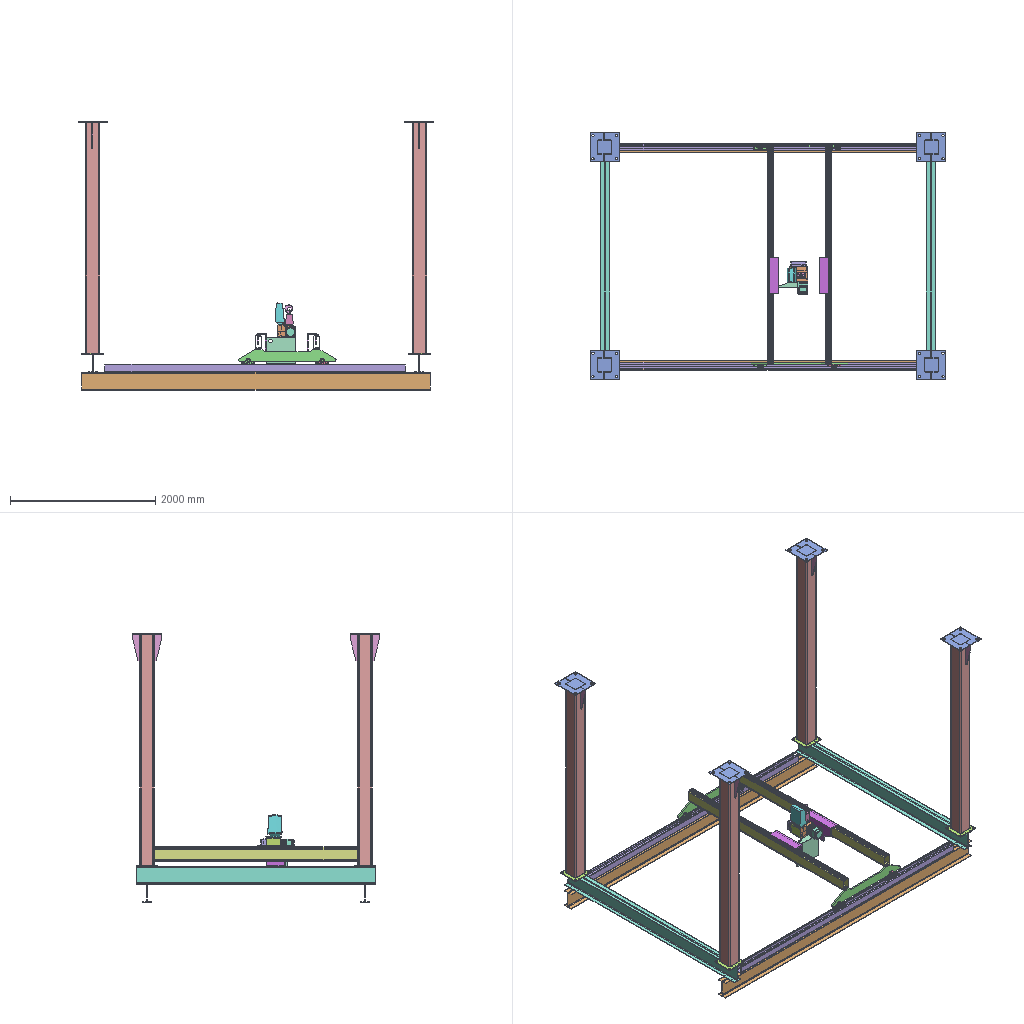Assembly | SolidWorks | 15 different items | 42 placed | box 4900 x 3400 x 3700 mm
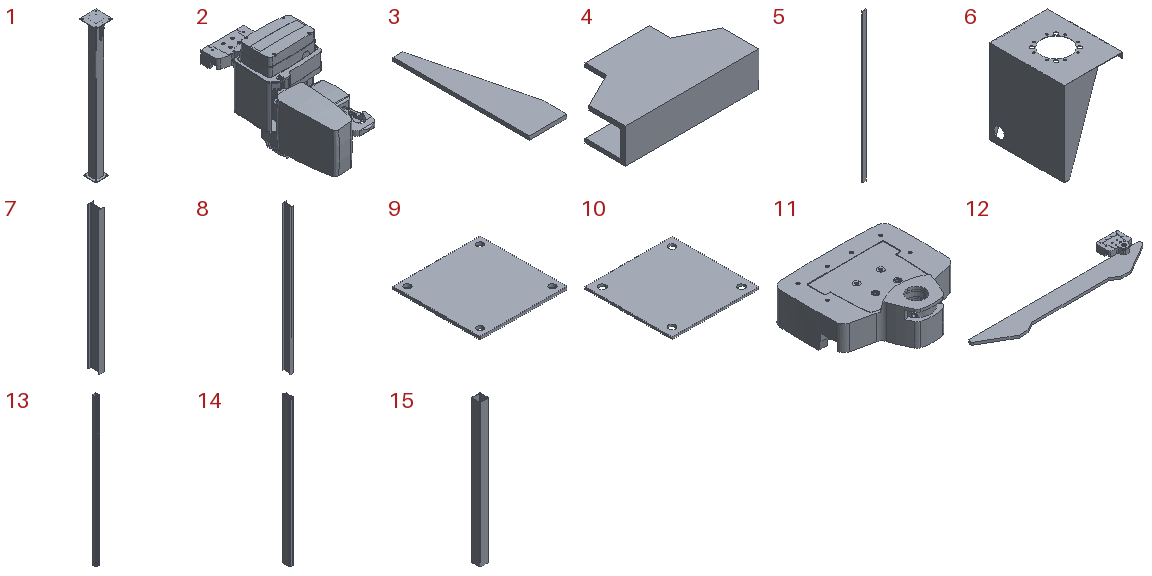Parts list (item | name | quantity | parent item | size | volume | features):
1 | (subassembly) | x4 | - | 400 x 400 x 3200 mm | 21789733 mm3 | -
2 | - | x1 | - | 284.321 x 680.473 x 459.6 mm | 19540266 mm3 | features BaseBody 17, ICE 1, Scale 1
3 | - | x8 | in 1 | 100 x 360 x 10 mm | 249000 mm3 | features Extrusion 1
4 | - | x2 | - | 500 x 280 x 130 mm | 3757451 mm3 | features ICE 2, Extrusion 1
5 | - | x2 | - | 70 x 14 x 3017 mm | 2956807 mm3 | features Extrusion 1
6 | - | x1 | - | 275 x 352 x 398 mm | 569864 mm3 | features ICE 4, Extrusion 1
7 | - | x2 | - | 125 x 250 x 3300 mm | 12199896 mm3 | features Extrusion 1
8 | - | x2 | - | 125 x 250 x 4800 mm | 17745303 mm3 | features Extrusion 1
9 | - | x4 | in 1 | 300 x 300 x 10 mm | 884795 mm3 | features Extrusion 1
10 | - | x4 | in 1 | 400 x 400 x 10 mm | 1567830 mm3 | features Extrusion 1
11 | - | x2 | - | 178.17 x 167.027 x 70 mm | 882482 mm3 | features BaseBody 1, Scale 1
12 | - | x2 | - | 1341 x 293.909 x 70 mm | 4218452 mm3 | features BaseBody 1, Fillet 1, ICE 1, Scale 1
13 | - | x2 | - | 100 x 110 x 4135 mm | 4470850 mm3 | features Extrusion 1
14 | - | x2 | - | 90 x 203.757 x 3017 mm | 5182605 mm3 | features Extrusion 1
15 | - | x4 | in 1 | 200 x 200 x 3180 mm | 18839108 mm3 | features Extrusion 1
Mates (type | each side: item.copy, entity, surface, feature):
In the top assembly
Coincident | 10.1 face plane Boss-Extrude1 | 10.2 face plane Boss-Extrude1 | 2 times
Coincident | 10.3 face plane Boss-Extrude1 | 10.1 face plane Boss-Extrude1 | 2 times
Coincident | 10.4 face plane Boss-Extrude1 | 10.3 face plane Boss-Extrude1 | 2 times
Coincident | 10.4 face plane Boss-Extrude1 | 10.2 face plane Boss-Extrude1
DistanceDim | 10.2 face plane Boss-Extrude1 | 10.4 face plane Boss-Extrude1
DistanceDim | 10.4 face plane Boss-Extrude1 | 10.3 face plane Boss-Extrude1
Coincident | 9.1 face plane Boss-Extrude1 | 7.1 face plane Boss-Extrude1 | 2 times
DistanceDim | 7.1 face plane Boss-Extrude1 | 9.1 face plane Boss-Extrude1
Coincident | 9.2 face plane Boss-Extrude1 | 7.2 face plane Boss-Extrude1 | 2 times
DistanceDim | 7.2 face plane Boss-Extrude1 | 9.2 face plane Boss-Extrude1
Coincident | 7.2 face plane Boss-Extrude1 | 8.1 face plane Boss-Extrude1
Coincident | 7.2 face plane Boss-Extrude1 | 8.2 face plane Boss-Extrude1
Coincident | 9.2 edge | 8.1 face plane Boss-Extrude1
Coincident | 9.3 face plane Boss-Extrude1 | 8.2 face plane Boss-Extrude1
DistanceDim | 8.1 face plane Boss-Extrude1 | 8.2 face plane Boss-Extrude1
DistanceDim | 8.1 face plane Boss-Extrude1 | 9.2 face plane Boss-Extrude1
Coincident | 8.1 face plane Boss-Extrude1 | 13.1 face plane Boss-Extrude1
DistanceDim | 13.1 face plane Boss-Extrude1 | 8.1 face plane Boss-Extrude1
DistanceDim | 13.1 face plane Boss-Extrude1 | 7.1 face plane Boss-Extrude1
Coincident | 12.1 face plane Seitenschild-RU22_34-1-solid1 | 11.1 face plane Seitenschild-RU22_34-1-solid1 | 2 times
DistanceDim | 11.1 edge | 12.1 edge
DistanceDim | 12.1 face plane Boss-Extrude1 | 13.1 face plane Boss-Extrude1 | 2 times
Coincident | 12.2 face plane Boss-Extrude1 | 5.1 face plane Boss-Extrude1 | 2 times
Coincident | 12.2 edge | 5.1 face plane Boss-Extrude1
Coincident | 12.2 face plane Boss-Extrude1 | 5.2 face plane Boss-Extrude1 | 2 times
Coincident | 12.2 edge | 5.2 face plane Boss-Extrude1
Coincident | 5.1 face plane Boss-Extrude1 | 14.1 face plane Boss-Extrude1 | 2 times
DistanceDim | 14.1 face plane Boss-Extrude1 | 5.1 face plane Boss-Extrude1
Coincident | 5.2 face plane Boss-Extrude1 | 14.2 face plane Boss-Extrude1
Coincident | 12.2 face plane Boss-Extrude1 | 14.2 face plane Boss-Extrude1
DistanceDim | 14.2 face plane Boss-Extrude1 | 5.2 face plane Boss-Extrude1
DistanceDim | 4.1 face plane Boss-Extrude3 | 14.1 face plane Boss-Extrude1
Coincident | 14.1 face plane Boss-Extrude1 | 4.1 face plane Boss-Extrude2
Coincident | 4.1 face plane Boss-Extrude1 | 4.2 face plane Boss-Extrude1 | 2 times
Coincident | 14.2 face plane Boss-Extrude1 | 4.2 face plane Boss-Extrude3
Coincident | 4.1 face plane Boss-Extrude1 | 6.1 face
DistanceDim | 6.1 face | 4.1 face plane Boss-Extrude1 | 2 times
Coincident | 6.1 face | 2.1 face plane Seitenschild-RU22_34-1-solid1
DistanceDim | 2.1 vertex | 10.3 face plane Boss-Extrude1
Parallel | 6.1 face | 2.1 face plane Cut-Extrude1
In subassembly 1
Coincident | 15.1 face plane Boss-Extrude1 | 10.5 face plane Boss-Extrude1
DistanceDim | 15.1 face plane Boss-Extrude1 | 10.5 face plane Boss-Extrude1 | 2 times
Coincident | 15.1 face plane Boss-Extrude1 | 9.4 face plane Boss-Extrude1
DistanceDim | 9.4 face plane Boss-Extrude1 | 15.1 face plane Boss-Extrude1 | 2 times
Coincident | 10.5 face plane Boss-Extrude1 | 3.1 face plane Boss-Extrude1
Coincident | 15.1 face plane Boss-Extrude1 | 3.1 face plane Boss-Extrude1
DistanceDim | 3.1 face plane Boss-Extrude1 | 10.5 face plane Boss-Extrude1
Coincident | 10.5 face plane Boss-Extrude1 | 3.2 face plane Boss-Extrude1
Coincident | 3.1 face plane Boss-Extrude1 | 3.2 face plane Boss-Extrude1
Coincident | 15.1 face plane Boss-Extrude1 | 3.2 face plane Boss-Extrude1